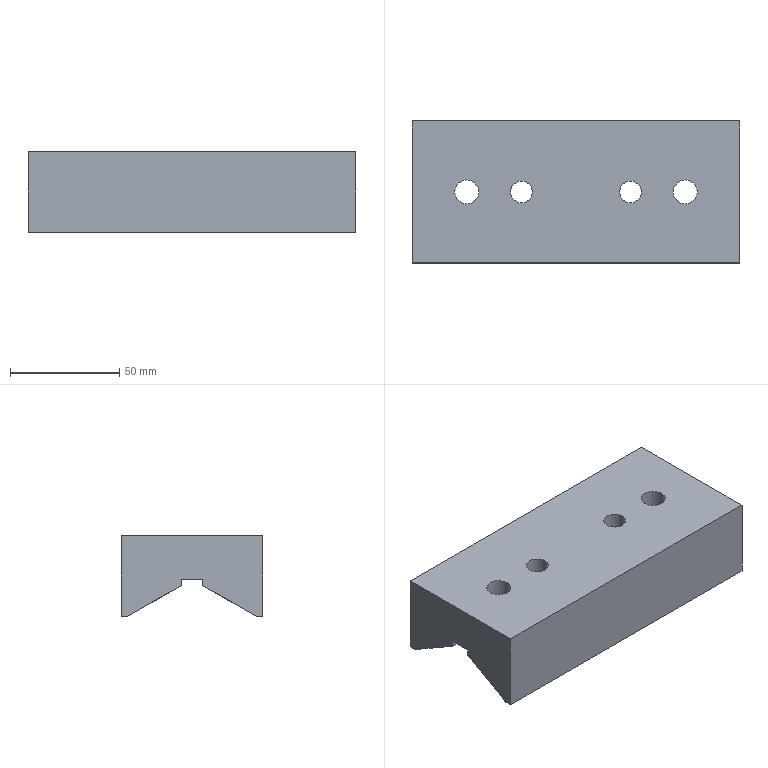Part | NX | features MAIN_BODY 2 | 1 solid | 34 faces | box 150 x 65 x 37 mm | volume 273059 mm3 | plane 24 | cylinder 10 | commonest cylinder face diameters 11 x6 10 x2 17.5 x2
STEP:
#1=CARTESIAN_POINT('',(625.,-5.,-355.));
#2=VERTEX_POINT('',#1);
#3=CARTESIAN_POINT('',(642.819,-5.,-355.));
#4=VERTEX_POINT('',#3);
#5=CARTESIAN_POINT('',(625.,-5.,-355.));
#6=DIRECTION('',(1.,0.,0.));
#7=VECTOR('',#6,1000.);
#8=LINE('',#5,#7);
#9=EDGE_CURVE('',#2,#4,#8,.T.);
#10=ORIENTED_EDGE('',*,*,#9,.F.);
#11=CARTESIAN_POINT('',(625.,5.,-355.));
#12=VERTEX_POINT('',#11);
#13=CARTESIAN_POINT('',(625.,5.,-355.));
#14=DIRECTION('',(0.,-1.,0.));
#15=VECTOR('',#14,1000.);
#16=LINE('',#13,#15);
#17=EDGE_CURVE('',#12,#2,#16,.T.);
#18=ORIENTED_EDGE('',*,*,#17,.F.);
#19=CARTESIAN_POINT('',(642.819,5.,-355.));
#20=VERTEX_POINT('',#19);
#21=CARTESIAN_POINT('',(625.,5.,-355.));
#22=DIRECTION('',(1.,0.,0.));
#23=VECTOR('',#22,1000.);
#24=LINE('',#21,#23);
#25=EDGE_CURVE('',#12,#20,#24,.T.);
#26=ORIENTED_EDGE('',*,*,#25,.T.);
#27=CARTESIAN_POINT('',(650.,0.,-355.));
#28=DIRECTION('',(0.,0.,-1.));
#29=DIRECTION('',(0.,-1.,0.));
#30=AXIS2_PLACEMENT_3D('',#27,#28,#29);
#31=CIRCLE('',#30,8.75);
#32=EDGE_CURVE('',#4,#20,#31,.T.);
#33=ORIENTED_EDGE('',*,*,#32,.F.);
#34=EDGE_LOOP('',(#10,#18,#26,#33));
#35=FACE_BOUND('',#34,.T.);
#36=CARTESIAN_POINT('',(625.,-5.,-355.));
#37=DIRECTION('',(0.,0.,1.));
#38=DIRECTION('',(0.,-1.,0.));
#39=AXIS2_PLACEMENT_3D('',#36,#37,#38);
#40=PLANE('',#39);
#41=ADVANCED_FACE('',(#35),#40,.F.);
#42=CARTESIAN_POINT('',(642.819,5.,-357.887));
#43=VERTEX_POINT('',#42);
#44=CARTESIAN_POINT('',(642.819,5.,-365.));
#45=DIRECTION('',(0.,0.,1.));
#46=VECTOR('',#45,1000.);
#47=LINE('',#44,#46);
#48=EDGE_CURVE('',#43,#20,#47,.T.);
#49=ORIENTED_EDGE('',*,*,#48,.T.);
#50=ORIENTED_EDGE('',*,*,#25,.F.);
#51=CARTESIAN_POINT('',(625.,5.,-357.887));
#52=VERTEX_POINT('',#51);
#53=CARTESIAN_POINT('',(625.,5.,-357.887));
#54=DIRECTION('',(0.,0.,1.));
#55=VECTOR('',#54,1000.);
#56=LINE('',#53,#55);
#57=EDGE_CURVE('',#52,#12,#56,.T.);
#58=ORIENTED_EDGE('',*,*,#57,.F.);
#59=CARTESIAN_POINT('',(625.,5.,-357.887));
#60=DIRECTION('',(1.,0.,0.));
#61=VECTOR('',#60,1000.);
#62=LINE('',#59,#61);
#63=EDGE_CURVE('',#52,#43,#62,.T.);
#64=ORIENTED_EDGE('',*,*,#63,.T.);
#65=EDGE_LOOP('',(#49,#50,#58,#64));
#66=FACE_BOUND('',#65,.T.);
#67=CARTESIAN_POINT('',(625.,5.,-357.887));
#68=DIRECTION('',(0.,-1.,0.));
#69=DIRECTION('',(0.,0.,-1.));
#70=AXIS2_PLACEMENT_3D('',#67,#68,#69);
#71=PLANE('',#70);
#72=ADVANCED_FACE('',(#66),#71,.T.);
#73=CARTESIAN_POINT('',(625.,-5.,-357.887));
#74=VERTEX_POINT('',#73);
#75=CARTESIAN_POINT('',(642.819,-5.,-357.887));
#76=VERTEX_POINT('',#75);
#77=CARTESIAN_POINT('',(625.,-5.,-357.887));
#78=DIRECTION('',(1.,0.,0.));
#79=VECTOR('',#78,1000.);
#80=LINE('',#77,#79);
#81=EDGE_CURVE('',#74,#76,#80,.T.);
#82=ORIENTED_EDGE('',*,*,#81,.F.);
#83=CARTESIAN_POINT('',(625.,-5.,-357.887));
#84=DIRECTION('',(0.,0.,1.));
#85=VECTOR('',#84,1000.);
#86=LINE('',#83,#85);
#87=EDGE_CURVE('',#74,#2,#86,.T.);
#88=ORIENTED_EDGE('',*,*,#87,.T.);
#89=ORIENTED_EDGE('',*,*,#9,.T.);
#90=CARTESIAN_POINT('',(642.819,-5.,-365.));
#91=DIRECTION('',(0.,0.,1.));
#92=VECTOR('',#91,1000.);
#93=LINE('',#90,#92);
#94=EDGE_CURVE('',#76,#4,#93,.T.);
#95=ORIENTED_EDGE('',*,*,#94,.F.);
#96=EDGE_LOOP('',(#82,#88,#89,#95));
#97=FACE_BOUND('',#96,.T.);
#98=CARTESIAN_POINT('',(625.,-5.,-357.887));
#99=DIRECTION('',(0.,-1.,0.));
#100=DIRECTION('',(0.,0.,-1.));
#101=AXIS2_PLACEMENT_3D('',#98,#99,#100);
#102=PLANE('',#101);
#103=ADVANCED_FACE('',(#97),#102,.F.);
#104=CARTESIAN_POINT('',(657.181,5.,-357.887));
#105=VERTEX_POINT('',#104);
#106=CARTESIAN_POINT('',(650.,0.,-355.));
#107=DIRECTION('',(0.,0.5,0.866));
#108=DIRECTION('',(0.,-0.866,0.5));
#109=AXIS2_PLACEMENT_3D('',#106,#107,#108);
#110=ELLIPSE('',#109,10.104,8.75);
#111=EDGE_CURVE('',#105,#43,#110,.T.);
#112=ORIENTED_EDGE('',*,*,#111,.T.);
#113=ORIENTED_EDGE('',*,*,#63,.F.);
#114=CARTESIAN_POINT('',(625.,29.445,-372.));
#115=VERTEX_POINT('',#114);
#116=CARTESIAN_POINT('',(625.,29.445,-372.));
#117=DIRECTION('',(0.,-0.866,0.5));
#118=VECTOR('',#117,1000.);
#119=LINE('',#116,#118);
#120=EDGE_CURVE('',#115,#52,#119,.T.);
#121=ORIENTED_EDGE('',*,*,#120,.F.);
#122=CARTESIAN_POINT('',(775.,29.445,-372.));
#123=VERTEX_POINT('',#122);
#124=CARTESIAN_POINT('',(625.,29.445,-372.));
#125=DIRECTION('',(1.,0.,0.));
#126=VECTOR('',#125,1000.);
#127=LINE('',#124,#126);
#128=EDGE_CURVE('',#115,#123,#127,.T.);
#129=ORIENTED_EDGE('',*,*,#128,.T.);
#130=CARTESIAN_POINT('',(775.,5.,-357.887));
#131=VERTEX_POINT('',#130);
#132=CARTESIAN_POINT('',(775.,29.445,-372.));
#133=DIRECTION('',(0.,-0.866,0.5));
#134=VECTOR('',#133,1000.);
#135=LINE('',#132,#134);
#136=EDGE_CURVE('',#123,#131,#135,.T.);
#137=ORIENTED_EDGE('',*,*,#136,.T.);
#138=CARTESIAN_POINT('',(757.181,5.,-357.887));
#139=VERTEX_POINT('',#138);
#140=CARTESIAN_POINT('',(625.,5.,-357.887));
#141=DIRECTION('',(1.,0.,0.));
#142=VECTOR('',#141,1000.);
#143=LINE('',#140,#142);
#144=EDGE_CURVE('',#139,#131,#143,.T.);
#145=ORIENTED_EDGE('',*,*,#144,.F.);
#146=CARTESIAN_POINT('',(742.819,5.,-357.887));
#147=VERTEX_POINT('',#146);
#148=CARTESIAN_POINT('',(750.,0.,-355.));
#149=DIRECTION('',(0.,0.5,0.866));
#150=DIRECTION('',(0.,-0.866,0.5));
#151=AXIS2_PLACEMENT_3D('',#148,#149,#150);
#152=ELLIPSE('',#151,10.104,8.75);
#153=EDGE_CURVE('',#147,#139,#152,.F.);
#154=ORIENTED_EDGE('',*,*,#153,.F.);
#155=CARTESIAN_POINT('',(727.291,5.,-357.887));
#156=VERTEX_POINT('',#155);
#157=CARTESIAN_POINT('',(625.,5.,-357.887));
#158=DIRECTION('',(1.,0.,0.));
#159=VECTOR('',#158,1000.);
#160=LINE('',#157,#159);
#161=EDGE_CURVE('',#156,#147,#160,.T.);
#162=ORIENTED_EDGE('',*,*,#161,.F.);
#163=CARTESIAN_POINT('',(722.709,5.,-357.887));
#164=VERTEX_POINT('',#163);
#165=CARTESIAN_POINT('',(725.,0.,-355.));
#166=DIRECTION('',(0.,0.5,0.866));
#167=DIRECTION('',(0.,0.866,-0.5));
#168=AXIS2_PLACEMENT_3D('',#165,#166,#167);
#169=ELLIPSE('',#168,6.351,5.5);
#170=EDGE_CURVE('',#164,#156,#169,.F.);
#171=ORIENTED_EDGE('',*,*,#170,.F.);
#172=CARTESIAN_POINT('',(677.291,5.,-357.887));
#173=VERTEX_POINT('',#172);
#174=CARTESIAN_POINT('',(625.,5.,-357.887));
#175=DIRECTION('',(1.,0.,0.));
#176=VECTOR('',#175,1000.);
#177=LINE('',#174,#176);
#178=EDGE_CURVE('',#173,#164,#177,.T.);
#179=ORIENTED_EDGE('',*,*,#178,.F.);
#180=CARTESIAN_POINT('',(672.709,5.,-357.887));
#181=VERTEX_POINT('',#180);
#182=CARTESIAN_POINT('',(675.,0.,-355.));
#183=DIRECTION('',(0.,0.5,0.866));
#184=DIRECTION('',(0.,0.866,-0.5));
#185=AXIS2_PLACEMENT_3D('',#182,#183,#184);
#186=ELLIPSE('',#185,6.351,5.5);
#187=EDGE_CURVE('',#181,#173,#186,.F.);
#188=ORIENTED_EDGE('',*,*,#187,.F.);
#189=CARTESIAN_POINT('',(625.,5.,-357.887));
#190=DIRECTION('',(1.,0.,0.));
#191=VECTOR('',#190,1000.);
#192=LINE('',#189,#191);
#193=EDGE_CURVE('',#105,#181,#192,.T.);
#194=ORIENTED_EDGE('',*,*,#193,.F.);
#195=EDGE_LOOP('',(#112,#113,#121,#129,#137,#145,#154,#162,#171,#179,#188,#194));
#196=FACE_BOUND('',#195,.T.);
#197=CARTESIAN_POINT('',(625.,29.445,-372.));
#198=DIRECTION('',(0.,-0.5,-0.866));
#199=DIRECTION('',(0.,0.866,-0.5));
#200=AXIS2_PLACEMENT_3D('',#197,#198,#199);
#201=PLANE('',#200);
#202=ADVANCED_FACE('',(#196),#201,.T.);
#203=CARTESIAN_POINT('',(727.291,5.,-355.));
#204=VERTEX_POINT('',#203);
#205=CARTESIAN_POINT('',(742.819,5.,-355.));
#206=VERTEX_POINT('',#205);
#207=CARTESIAN_POINT('',(625.,5.,-355.));
#208=DIRECTION('',(1.,0.,0.));
#209=VECTOR('',#208,1000.);
#210=LINE('',#207,#209);
#211=EDGE_CURVE('',#204,#206,#210,.T.);
#212=ORIENTED_EDGE('',*,*,#211,.F.);
#213=CARTESIAN_POINT('',(727.291,5.,-355.));
#214=DIRECTION('',(0.,0.,-1.));
#215=VECTOR('',#214,1000.);
#216=LINE('',#213,#215);
#217=EDGE_CURVE('',#156,#204,#216,.F.);
#218=ORIENTED_EDGE('',*,*,#217,.F.);
#219=ORIENTED_EDGE('',*,*,#161,.T.);
#220=CARTESIAN_POINT('',(742.819,5.,-365.));
#221=DIRECTION('',(0.,0.,1.));
#222=VECTOR('',#221,1000.);
#223=LINE('',#220,#222);
#224=EDGE_CURVE('',#206,#147,#223,.F.);
#225=ORIENTED_EDGE('',*,*,#224,.F.);
#226=EDGE_LOOP('',(#212,#218,#219,#225));
#227=FACE_BOUND('',#226,.T.);
#228=CARTESIAN_POINT('',(625.,5.,-357.887));
#229=DIRECTION('',(0.,-1.,0.));
#230=DIRECTION('',(0.,0.,-1.));
#231=AXIS2_PLACEMENT_3D('',#228,#229,#230);
#232=PLANE('',#231);
#233=ADVANCED_FACE('',(#227),#232,.T.);
#234=ORIENTED_EDGE('',*,*,#144,.T.);
#235=CARTESIAN_POINT('',(775.,5.,-355.));
#236=VERTEX_POINT('',#235);
#237=CARTESIAN_POINT('',(775.,5.,-357.887));
#238=DIRECTION('',(0.,0.,1.));
#239=VECTOR('',#238,1000.);
#240=LINE('',#237,#239);
#241=EDGE_CURVE('',#131,#236,#240,.T.);
#242=ORIENTED_EDGE('',*,*,#241,.T.);
#243=CARTESIAN_POINT('',(757.181,5.,-355.));
#244=VERTEX_POINT('',#243);
#245=CARTESIAN_POINT('',(625.,5.,-355.));
#246=DIRECTION('',(1.,0.,0.));
#247=VECTOR('',#246,1000.);
#248=LINE('',#245,#247);
#249=EDGE_CURVE('',#244,#236,#248,.T.);
#250=ORIENTED_EDGE('',*,*,#249,.F.);
#251=CARTESIAN_POINT('',(757.181,5.,-365.));
#252=DIRECTION('',(0.,0.,1.));
#253=VECTOR('',#252,1000.);
#254=LINE('',#251,#253);
#255=EDGE_CURVE('',#139,#244,#254,.T.);
#256=ORIENTED_EDGE('',*,*,#255,.F.);
#257=EDGE_LOOP('',(#234,#242,#250,#256));
#258=FACE_BOUND('',#257,.T.);
#259=CARTESIAN_POINT('',(625.,5.,-357.887));
#260=DIRECTION('',(0.,-1.,0.));
#261=DIRECTION('',(0.,0.,-1.));
#262=AXIS2_PLACEMENT_3D('',#259,#260,#261);
#263=PLANE('',#262);
#264=ADVANCED_FACE('',(#258),#263,.T.);
#265=CARTESIAN_POINT('',(742.819,-5.,-355.));
#266=VERTEX_POINT('',#265);
#267=CARTESIAN_POINT('',(742.819,-5.,-357.887));
#268=VERTEX_POINT('',#267);
#269=CARTESIAN_POINT('',(742.819,-5.,-365.));
#270=DIRECTION('',(0.,0.,1.));
#271=VECTOR('',#270,1000.);
#272=LINE('',#269,#271);
#273=EDGE_CURVE('',#266,#268,#272,.F.);
#274=ORIENTED_EDGE('',*,*,#273,.T.);
#275=CARTESIAN_POINT('',(727.291,-5.,-357.887));
#276=VERTEX_POINT('',#275);
#277=CARTESIAN_POINT('',(625.,-5.,-357.887));
#278=DIRECTION('',(1.,0.,0.));
#279=VECTOR('',#278,1000.);
#280=LINE('',#277,#279);
#281=EDGE_CURVE('',#276,#268,#280,.T.);
#282=ORIENTED_EDGE('',*,*,#281,.F.);
#283=CARTESIAN_POINT('',(727.291,-5.,-355.));
#284=VERTEX_POINT('',#283);
#285=CARTESIAN_POINT('',(727.291,-5.,-355.));
#286=DIRECTION('',(0.,0.,-1.));
#287=VECTOR('',#286,1000.);
#288=LINE('',#285,#287);
#289=EDGE_CURVE('',#276,#284,#288,.F.);
#290=ORIENTED_EDGE('',*,*,#289,.T.);
#291=CARTESIAN_POINT('',(625.,-5.,-355.));
#292=DIRECTION('',(1.,0.,0.));
#293=VECTOR('',#292,1000.);
#294=LINE('',#291,#293);
#295=EDGE_CURVE('',#284,#266,#294,.T.);
#296=ORIENTED_EDGE('',*,*,#295,.T.);
#297=EDGE_LOOP('',(#274,#282,#290,#296));
#298=FACE_BOUND('',#297,.T.);
#299=CARTESIAN_POINT('',(625.,-5.,-357.887));
#300=DIRECTION('',(0.,-1.,0.));
#301=DIRECTION('',(0.,0.,-1.));
#302=AXIS2_PLACEMENT_3D('',#299,#300,#301);
#303=PLANE('',#302);
#304=ADVANCED_FACE('',(#298),#303,.F.);
#305=CARTESIAN_POINT('',(757.181,-5.,-357.887));
#306=VERTEX_POINT('',#305);
#307=CARTESIAN_POINT('',(757.181,-5.,-355.));
#308=VERTEX_POINT('',#307);
#309=CARTESIAN_POINT('',(757.181,-5.,-365.));
#310=DIRECTION('',(0.,0.,1.));
#311=VECTOR('',#310,1000.);
#312=LINE('',#309,#311);
#313=EDGE_CURVE('',#306,#308,#312,.T.);
#314=ORIENTED_EDGE('',*,*,#313,.T.);
#315=CARTESIAN_POINT('',(775.,-5.,-355.));
#316=VERTEX_POINT('',#315);
#317=CARTESIAN_POINT('',(625.,-5.,-355.));
#318=DIRECTION('',(1.,0.,0.));
#319=VECTOR('',#318,1000.);
#320=LINE('',#317,#319);
#321=EDGE_CURVE('',#308,#316,#320,.T.);
#322=ORIENTED_EDGE('',*,*,#321,.T.);
#323=CARTESIAN_POINT('',(775.,-5.,-357.887));
#324=VERTEX_POINT('',#323);
#325=CARTESIAN_POINT('',(775.,-5.,-357.887));
#326=DIRECTION('',(0.,0.,1.));
#327=VECTOR('',#326,1000.);
#328=LINE('',#325,#327);
#329=EDGE_CURVE('',#324,#316,#328,.T.);
#330=ORIENTED_EDGE('',*,*,#329,.F.);
#331=CARTESIAN_POINT('',(625.,-5.,-357.887));
#332=DIRECTION('',(1.,0.,0.));
#333=VECTOR('',#332,1000.);
#334=LINE('',#331,#333);
#335=EDGE_CURVE('',#306,#324,#334,.T.);
#336=ORIENTED_EDGE('',*,*,#335,.F.);
#337=EDGE_LOOP('',(#314,#322,#330,#336));
#338=FACE_BOUND('',#337,.T.);
#339=CARTESIAN_POINT('',(625.,-5.,-357.887));
#340=DIRECTION('',(0.,-1.,0.));
#341=DIRECTION('',(0.,0.,-1.));
#342=AXIS2_PLACEMENT_3D('',#339,#340,#341);
#343=PLANE('',#342);
#344=ADVANCED_FACE('',(#338),#343,.F.);
#345=CARTESIAN_POINT('',(657.181,-5.,-357.887));
#346=VERTEX_POINT('',#345);
#347=CARTESIAN_POINT('',(672.709,-5.,-357.887));
#348=VERTEX_POINT('',#347);
#349=CARTESIAN_POINT('',(625.,-5.,-357.887));
#350=DIRECTION('',(1.,0.,0.));
#351=VECTOR('',#350,1000.);
#352=LINE('',#349,#351);
#353=EDGE_CURVE('',#346,#348,#352,.T.);
#354=ORIENTED_EDGE('',*,*,#353,.T.);
#355=CARTESIAN_POINT('',(677.291,-5.,-357.887));
#356=VERTEX_POINT('',#355);
#357=CARTESIAN_POINT('',(675.,0.,-355.));
#358=DIRECTION('',(0.,0.5,-0.866));
#359=DIRECTION('',(0.,-0.866,-0.5));
#360=AXIS2_PLACEMENT_3D('',#357,#358,#359);
#361=ELLIPSE('',#360,6.351,5.5);
#362=EDGE_CURVE('',#348,#356,#361,.F.);
#363=ORIENTED_EDGE('',*,*,#362,.T.);
#364=CARTESIAN_POINT('',(722.709,-5.,-357.887));
#365=VERTEX_POINT('',#364);
#366=CARTESIAN_POINT('',(625.,-5.,-357.887));
#367=DIRECTION('',(1.,0.,0.));
#368=VECTOR('',#367,1000.);
#369=LINE('',#366,#368);
#370=EDGE_CURVE('',#356,#365,#369,.T.);
#371=ORIENTED_EDGE('',*,*,#370,.T.);
#372=CARTESIAN_POINT('',(725.,0.,-355.));
#373=DIRECTION('',(0.,0.5,-0.866));
#374=DIRECTION('',(0.,-0.866,-0.5));
#375=AXIS2_PLACEMENT_3D('',#372,#373,#374);
#376=ELLIPSE('',#375,6.351,5.5);
#377=EDGE_CURVE('',#365,#276,#376,.F.);
#378=ORIENTED_EDGE('',*,*,#377,.T.);
#379=ORIENTED_EDGE('',*,*,#281,.T.);
#380=CARTESIAN_POINT('',(750.,0.,-355.));
#381=DIRECTION('',(0.,0.5,-0.866));
#382=DIRECTION('',(0.,0.866,0.5));
#383=AXIS2_PLACEMENT_3D('',#380,#381,#382);
#384=ELLIPSE('',#383,10.104,8.75);
#385=EDGE_CURVE('',#268,#306,#384,.F.);
#386=ORIENTED_EDGE('',*,*,#385,.T.);
#387=ORIENTED_EDGE('',*,*,#335,.T.);
#388=CARTESIAN_POINT('',(775.,-29.445,-372.));
#389=VERTEX_POINT('',#388);
#390=CARTESIAN_POINT('',(775.,-29.445,-372.));
#391=DIRECTION('',(0.,0.866,0.5));
#392=VECTOR('',#391,1000.);
#393=LINE('',#390,#392);
#394=EDGE_CURVE('',#389,#324,#393,.T.);
#395=ORIENTED_EDGE('',*,*,#394,.F.);
#396=CARTESIAN_POINT('',(625.,-29.445,-372.));
#397=VERTEX_POINT('',#396);
#398=CARTESIAN_POINT('',(625.,-29.445,-372.));
#399=DIRECTION('',(1.,0.,0.));
#400=VECTOR('',#399,1000.);
#401=LINE('',#398,#400);
#402=EDGE_CURVE('',#397,#389,#401,.T.);
#403=ORIENTED_EDGE('',*,*,#402,.F.);
#404=CARTESIAN_POINT('',(625.,-29.445,-372.));
#405=DIRECTION('',(0.,0.866,0.5));
#406=VECTOR('',#405,1000.);
#407=LINE('',#404,#406);
#408=EDGE_CURVE('',#397,#74,#407,.T.);
#409=ORIENTED_EDGE('',*,*,#408,.T.);
#410=ORIENTED_EDGE('',*,*,#81,.T.);
#411=CARTESIAN_POINT('',(650.,0.,-355.));
#412=DIRECTION('',(0.,0.5,-0.866));
#413=DIRECTION('',(0.,0.866,0.5));
#414=AXIS2_PLACEMENT_3D('',#411,#412,#413);
#415=ELLIPSE('',#414,10.104,8.75);
#416=EDGE_CURVE('',#346,#76,#415,.T.);
#417=ORIENTED_EDGE('',*,*,#416,.F.);
#418=EDGE_LOOP('',(#354,#363,#371,#378,#379,#386,#387,#395,#403,#409,#410,#417));
#419=FACE_BOUND('',#418,.T.);
#420=CARTESIAN_POINT('',(625.,-29.445,-372.));
#421=DIRECTION('',(0.,-0.5,0.866));
#422=DIRECTION('',(0.,-0.866,-0.5));
#423=AXIS2_PLACEMENT_3D('',#420,#421,#422);
#424=PLANE('',#423);
#425=ADVANCED_FACE('',(#419),#424,.F.);
#426=CARTESIAN_POINT('',(750.,0.,-355.));
#427=DIRECTION('',(0.,0.,-1.));
#428=DIRECTION('',(0.,-1.,0.));
#429=AXIS2_PLACEMENT_3D('',#426,#427,#428);
#430=CIRCLE('',#429,8.75);
#431=EDGE_CURVE('',#308,#244,#430,.F.);
#432=ORIENTED_EDGE('',*,*,#431,.T.);
#433=ORIENTED_EDGE('',*,*,#249,.T.);
#434=CARTESIAN_POINT('',(775.,-5.,-355.));
#435=DIRECTION('',(0.,1.,0.));
#436=VECTOR('',#435,1000.);
#437=LINE('',#434,#436);
#438=EDGE_CURVE('',#316,#236,#437,.T.);
#439=ORIENTED_EDGE('',*,*,#438,.F.);
#440=ORIENTED_EDGE('',*,*,#321,.F.);
#441=EDGE_LOOP('',(#432,#433,#439,#440));
#442=FACE_BOUND('',#441,.T.);
#443=CARTESIAN_POINT('',(625.,-5.,-355.));
#444=DIRECTION('',(0.,0.,1.));
#445=DIRECTION('',(0.,-1.,0.));
#446=AXIS2_PLACEMENT_3D('',#443,#444,#445);
#447=PLANE('',#446);
#448=ADVANCED_FACE('',(#442),#447,.F.);
#449=CARTESIAN_POINT('',(675.,5.,-355.));
#450=VERTEX_POINT('',#449);
#451=CARTESIAN_POINT('',(675.,0.,-355.));
#452=DIRECTION('',(0.,0.,1.));
#453=DIRECTION('',(0.,1.,0.));
#454=AXIS2_PLACEMENT_3D('',#451,#452,#453);
#455=CIRCLE('',#454,5.);
#456=EDGE_CURVE('',#450,#450,#455,.T.);
#457=ORIENTED_EDGE('',*,*,#456,.T.);
#458=EDGE_LOOP('',(#457));
#459=FACE_BOUND('',#458,.T.);
#460=CARTESIAN_POINT('',(725.,5.,-355.));
#461=VERTEX_POINT('',#460);
#462=CARTESIAN_POINT('',(725.,0.,-355.));
#463=DIRECTION('',(0.,0.,1.));
#464=DIRECTION('',(0.,1.,0.));
#465=AXIS2_PLACEMENT_3D('',#462,#463,#464);
#466=CIRCLE('',#465,5.);
#467=EDGE_CURVE('',#461,#461,#466,.T.);
#468=ORIENTED_EDGE('',*,*,#467,.T.);
#469=EDGE_LOOP('',(#468));
#470=FACE_BOUND('',#469,.T.);
#471=CARTESIAN_POINT('',(657.181,5.,-355.));
#472=VERTEX_POINT('',#471);
#473=CARTESIAN_POINT('',(672.709,5.,-355.));
#474=VERTEX_POINT('',#473);
#475=CARTESIAN_POINT('',(625.,5.,-355.));
#476=DIRECTION('',(1.,0.,0.));
#477=VECTOR('',#476,1000.);
#478=LINE('',#475,#477);
#479=EDGE_CURVE('',#472,#474,#478,.T.);
#480=ORIENTED_EDGE('',*,*,#479,.T.);
#481=CARTESIAN_POINT('',(677.291,5.,-355.));
#482=VERTEX_POINT('',#481);
#483=CARTESIAN_POINT('',(675.,0.,-355.));
#484=DIRECTION('',(0.,0.,1.));
#485=DIRECTION('',(0.,1.,0.));
#486=AXIS2_PLACEMENT_3D('',#483,#484,#485);
#487=CIRCLE('',#486,5.5);
#488=EDGE_CURVE('',#474,#482,#487,.F.);
#489=ORIENTED_EDGE('',*,*,#488,.T.);
#490=CARTESIAN_POINT('',(722.709,5.,-355.));
#491=VERTEX_POINT('',#490);
#492=CARTESIAN_POINT('',(625.,5.,-355.));
#493=DIRECTION('',(1.,0.,0.));
#494=VECTOR('',#493,1000.);
#495=LINE('',#492,#494);
#496=EDGE_CURVE('',#482,#491,#495,.T.);
#497=ORIENTED_EDGE('',*,*,#496,.T.);
#498=CARTESIAN_POINT('',(725.,0.,-355.));
#499=DIRECTION('',(0.,0.,1.));
#500=DIRECTION('',(0.,1.,0.));
#501=AXIS2_PLACEMENT_3D('',#498,#499,#500);
#502=CIRCLE('',#501,5.5);
#503=EDGE_CURVE('',#491,#204,#502,.F.);
#504=ORIENTED_EDGE('',*,*,#503,.T.);
#505=ORIENTED_EDGE('',*,*,#211,.T.);
#506=CARTESIAN_POINT('',(750.,0.,-355.));
#507=DIRECTION('',(0.,0.,-1.));
#508=DIRECTION('',(0.,-1.,0.));
#509=AXIS2_PLACEMENT_3D('',#506,#507,#508);
#510=CIRCLE('',#509,8.75);
#511=EDGE_CURVE('',#206,#266,#510,.F.);
#512=ORIENTED_EDGE('',*,*,#511,.T.);
#513=ORIENTED_EDGE('',*,*,#295,.F.);
#514=CARTESIAN_POINT('',(722.709,-5.,-355.));
#515=VERTEX_POINT('',#514);
#516=CARTESIAN_POINT('',(725.,0.,-355.));
#517=DIRECTION('',(0.,0.,1.));
#518=DIRECTION('',(0.,1.,0.));
#519=AXIS2_PLACEMENT_3D('',#516,#517,#518);
#520=CIRCLE('',#519,5.5);
#521=EDGE_CURVE('',#284,#515,#520,.F.);
#522=ORIENTED_EDGE('',*,*,#521,.T.);
#523=CARTESIAN_POINT('',(677.291,-5.,-355.));
#524=VERTEX_POINT('',#523);
#525=CARTESIAN_POINT('',(625.,-5.,-355.));
#526=DIRECTION('',(1.,0.,0.));
#527=VECTOR('',#526,1000.);
#528=LINE('',#525,#527);
#529=EDGE_CURVE('',#524,#515,#528,.T.);
#530=ORIENTED_EDGE('',*,*,#529,.F.);
#531=CARTESIAN_POINT('',(672.709,-5.,-355.));
#532=VERTEX_POINT('',#531);
#533=CARTESIAN_POINT('',(675.,0.,-355.));
#534=DIRECTION('',(0.,0.,1.));
#535=DIRECTION('',(0.,1.,0.));
#536=AXIS2_PLACEMENT_3D('',#533,#534,#535);
#537=CIRCLE('',#536,5.5);
#538=EDGE_CURVE('',#524,#532,#537,.F.);
#539=ORIENTED_EDGE('',*,*,#538,.T.);
#540=CARTESIAN_POINT('',(657.181,-5.,-355.));
#541=VERTEX_POINT('',#540);
#542=CARTESIAN_POINT('',(625.,-5.,-355.));
#543=DIRECTION('',(1.,0.,0.));
#544=VECTOR('',#543,1000.);
#545=LINE('',#542,#544);
#546=EDGE_CURVE('',#541,#532,#545,.T.);
#547=ORIENTED_EDGE('',*,*,#546,.F.);
#548=CARTESIAN_POINT('',(650.,0.,-355.));
#549=DIRECTION('',(0.,0.,-1.));
#550=DIRECTION('',(0.,-1.,0.));
#551=AXIS2_PLACEMENT_3D('',#548,#549,#550);
#552=CIRCLE('',#551,8.75);
#553=EDGE_CURVE('',#472,#541,#552,.T.);
#554=ORIENTED_EDGE('',*,*,#553,.F.);
#555=EDGE_LOOP('',(#480,#489,#497,#504,#505,#512,#513,#522,#530,#539,#547,#554));
#556=FACE_BOUND('',#555,.T.);
#557=CARTESIAN_POINT('',(625.,-5.,-355.));
#558=DIRECTION('',(0.,0.,1.));
#559=DIRECTION('',(0.,-1.,0.));
#560=AXIS2_PLACEMENT_3D('',#557,#558,#559);
#561=PLANE('',#560);
#562=ADVANCED_FACE('',(#459,#470,#556),#561,.F.);
#563=CARTESIAN_POINT('',(650.,5.5,-335.));
#564=VERTEX_POINT('',#563);
#565=CARTESIAN_POINT('',(650.,0.,-335.));
#566=DIRECTION('',(0.,0.,-1.));
#567=DIRECTION('',(0.,1.,0.));
#568=AXIS2_PLACEMENT_3D('',#565,#566,#567);
#569=CIRCLE('',#568,5.5);
#570=EDGE_CURVE('',#564,#564,#569,.T.);
#571=ORIENTED_EDGE('',*,*,#570,.T.);
#572=EDGE_LOOP('',(#571));
#573=FACE_BOUND('',#572,.T.);
#574=CARTESIAN_POINT('',(775.,-32.5,-335.));
#575=VERTEX_POINT('',#574);
#576=CARTESIAN_POINT('',(775.,32.5,-335.));
#577=VERTEX_POINT('',#576);
#578=CARTESIAN_POINT('',(775.,0.,-335.));
#579=DIRECTION('',(0.,1.,0.));
#580=VECTOR('',#579,1000.);
#581=LINE('',#578,#580);
#582=EDGE_CURVE('',#575,#577,#581,.T.);
#583=ORIENTED_EDGE('',*,*,#582,.T.);
#584=CARTESIAN_POINT('',(625.,32.5,-335.));
#585=VERTEX_POINT('',#584);
#586=CARTESIAN_POINT('',(625.,32.5,-335.));
#587=DIRECTION('',(1.,0.,0.));
#588=VECTOR('',#587,1000.);
#589=LINE('',#586,#588);
#590=EDGE_CURVE('',#585,#577,#589,.T.);
#591=ORIENTED_EDGE('',*,*,#590,.F.);
#592=CARTESIAN_POINT('',(625.,-32.5,-335.));
#593=VERTEX_POINT('',#592);
#594=CARTESIAN_POINT('',(625.,0.,-335.));
#595=DIRECTION('',(0.,-1.,0.));
#596=VECTOR('',#595,1000.);
#597=LINE('',#594,#596);
#598=EDGE_CURVE('',#585,#593,#597,.T.);
#599=ORIENTED_EDGE('',*,*,#598,.T.);
#600=CARTESIAN_POINT('',(625.,-32.5,-335.));
#601=DIRECTION('',(1.,0.,0.));
#602=VECTOR('',#601,1000.);
#603=LINE('',#600,#602);
#604=EDGE_CURVE('',#593,#575,#603,.T.);
#605=ORIENTED_EDGE('',*,*,#604,.T.);
#606=EDGE_LOOP('',(#583,#591,#599,#605));
#607=FACE_BOUND('',#606,.T.);
#608=CARTESIAN_POINT('',(675.,5.,-335.));
#609=VERTEX_POINT('',#608);
#610=CARTESIAN_POINT('',(675.,0.,-335.));
#611=DIRECTION('',(0.,0.,1.));
#612=DIRECTION('',(0.,1.,0.));
#613=AXIS2_PLACEMENT_3D('',#610,#611,#612);
#614=CIRCLE('',#613,5.);
#615=EDGE_CURVE('',#609,#609,#614,.T.);
#616=ORIENTED_EDGE('',*,*,#615,.F.);
#617=EDGE_LOOP('',(#616));
#618=FACE_BOUND('',#617,.T.);
#619=CARTESIAN_POINT('',(725.,5.,-335.));
#620=VERTEX_POINT('',#619);
#621=CARTESIAN_POINT('',(725.,0.,-335.));
#622=DIRECTION('',(0.,0.,1.));
#623=DIRECTION('',(0.,1.,0.));
#624=AXIS2_PLACEMENT_3D('',#621,#622,#623);
#625=CIRCLE('',#624,5.);
#626=EDGE_CURVE('',#620,#620,#625,.T.);
#627=ORIENTED_EDGE('',*,*,#626,.F.);
#628=EDGE_LOOP('',(#627));
#629=FACE_BOUND('',#628,.T.);
#630=CARTESIAN_POINT('',(750.,5.5,-335.));
#631=VERTEX_POINT('',#630);
#632=CARTESIAN_POINT('',(750.,0.,-335.));
#633=DIRECTION('',(0.,0.,1.));
#634=DIRECTION('',(0.,1.,0.));
#635=AXIS2_PLACEMENT_3D('',#632,#633,#634);
#636=CIRCLE('',#635,5.5);
#637=EDGE_CURVE('',#631,#631,#636,.T.);
#638=ORIENTED_EDGE('',*,*,#637,.F.);
#639=EDGE_LOOP('',(#638));
#640=FACE_BOUND('',#639,.T.);
#641=CARTESIAN_POINT('',(625.,0.,-335.));
#642=DIRECTION('',(0.,0.,1.));
#643=DIRECTION('',(0.,-1.,0.));
#644=AXIS2_PLACEMENT_3D('',#641,#642,#643);
#645=PLANE('',#644);
#646=ADVANCED_FACE('',(#573,#607,#618,#629,#640),#645,.T.);
#647=ORIENTED_EDGE('',*,*,#496,.F.);
#648=CARTESIAN_POINT('',(677.291,5.,-355.));
#649=DIRECTION('',(0.,0.,-1.));
#650=VECTOR('',#649,1000.);
#651=LINE('',#648,#650);
#652=EDGE_CURVE('',#173,#482,#651,.F.);
#653=ORIENTED_EDGE('',*,*,#652,.F.);
#654=ORIENTED_EDGE('',*,*,#178,.T.);
#655=CARTESIAN_POINT('',(722.709,5.,-355.));
#656=DIRECTION('',(0.,0.,-1.));
#657=VECTOR('',#656,1000.);
#658=LINE('',#655,#657);
#659=EDGE_CURVE('',#491,#164,#658,.T.);
#660=ORIENTED_EDGE('',*,*,#659,.F.);
#661=EDGE_LOOP('',(#647,#653,#654,#660));
#662=FACE_BOUND('',#661,.T.);
#663=CARTESIAN_POINT('',(625.,5.,-357.887));
#664=DIRECTION('',(0.,-1.,0.));
#665=DIRECTION('',(0.,0.,-1.));
#666=AXIS2_PLACEMENT_3D('',#663,#664,#665);
#667=PLANE('',#666);
#668=ADVANCED_FACE('',(#662),#667,.T.);
#669=CARTESIAN_POINT('',(722.709,-5.,-355.));
#670=DIRECTION('',(0.,0.,-1.));
#671=VECTOR('',#670,1000.);
#672=LINE('',#669,#671);
#673=EDGE_CURVE('',#515,#365,#672,.T.);
#674=ORIENTED_EDGE('',*,*,#673,.T.);
#675=ORIENTED_EDGE('',*,*,#370,.F.);
#676=CARTESIAN_POINT('',(677.291,-5.,-355.));
#677=DIRECTION('',(0.,0.,-1.));
#678=VECTOR('',#677,1000.);
#679=LINE('',#676,#678);
#680=EDGE_CURVE('',#356,#524,#679,.F.);
#681=ORIENTED_EDGE('',*,*,#680,.T.);
#682=ORIENTED_EDGE('',*,*,#529,.T.);
#683=EDGE_LOOP('',(#674,#675,#681,#682));
#684=FACE_BOUND('',#683,.T.);
#685=CARTESIAN_POINT('',(625.,-5.,-357.887));
#686=DIRECTION('',(0.,-1.,0.));
#687=DIRECTION('',(0.,0.,-1.));
#688=AXIS2_PLACEMENT_3D('',#685,#686,#687);
#689=PLANE('',#688);
#690=ADVANCED_FACE('',(#684),#689,.F.);
#691=CARTESIAN_POINT('',(657.181,5.,-365.));
#692=DIRECTION('',(0.,0.,1.));
#693=VECTOR('',#692,1000.);
#694=LINE('',#691,#693);
#695=EDGE_CURVE('',#472,#105,#694,.F.);
#696=ORIENTED_EDGE('',*,*,#695,.T.);
#697=ORIENTED_EDGE('',*,*,#193,.T.);
#698=CARTESIAN_POINT('',(672.709,5.,-355.));
#699=DIRECTION('',(0.,0.,-1.));
#700=VECTOR('',#699,1000.);
#701=LINE('',#698,#700);
#702=EDGE_CURVE('',#474,#181,#701,.T.);
#703=ORIENTED_EDGE('',*,*,#702,.F.);
#704=ORIENTED_EDGE('',*,*,#479,.F.);
#705=EDGE_LOOP('',(#696,#697,#703,#704));
#706=FACE_BOUND('',#705,.T.);
#707=CARTESIAN_POINT('',(625.,5.,-357.887));
#708=DIRECTION('',(0.,-1.,0.));
#709=DIRECTION('',(0.,0.,-1.));
#710=AXIS2_PLACEMENT_3D('',#707,#708,#709);
#711=PLANE('',#710);
#712=ADVANCED_FACE('',(#706),#711,.T.);
#713=ORIENTED_EDGE('',*,*,#546,.T.);
#714=CARTESIAN_POINT('',(672.709,-5.,-355.));
#715=DIRECTION('',(0.,0.,-1.));
#716=VECTOR('',#715,1000.);
#717=LINE('',#714,#716);
#718=EDGE_CURVE('',#532,#348,#717,.T.);
#719=ORIENTED_EDGE('',*,*,#718,.T.);
#720=ORIENTED_EDGE('',*,*,#353,.F.);
#721=CARTESIAN_POINT('',(657.181,-5.,-365.));
#722=DIRECTION('',(0.,0.,1.));
#723=VECTOR('',#722,1000.);
#724=LINE('',#721,#723);
#725=EDGE_CURVE('',#541,#346,#724,.F.);
#726=ORIENTED_EDGE('',*,*,#725,.F.);
#727=EDGE_LOOP('',(#713,#719,#720,#726));
#728=FACE_BOUND('',#727,.T.);
#729=CARTESIAN_POINT('',(625.,-5.,-357.887));
#730=DIRECTION('',(0.,-1.,0.));
#731=DIRECTION('',(0.,0.,-1.));
#732=AXIS2_PLACEMENT_3D('',#729,#730,#731);
#733=PLANE('',#732);
#734=ADVANCED_FACE('',(#728),#733,.F.);
#735=CARTESIAN_POINT('',(775.,32.5,-372.));
#736=VERTEX_POINT('',#735);
#737=CARTESIAN_POINT('',(775.,32.5,-372.));
#738=DIRECTION('',(0.,-1.,0.));
#739=VECTOR('',#738,1000.);
#740=LINE('',#737,#739);
#741=EDGE_CURVE('',#736,#123,#740,.T.);
#742=ORIENTED_EDGE('',*,*,#741,.T.);
#743=ORIENTED_EDGE('',*,*,#128,.F.);
#744=CARTESIAN_POINT('',(625.,32.5,-372.));
#745=VERTEX_POINT('',#744);
#746=CARTESIAN_POINT('',(625.,32.5,-372.));
#747=DIRECTION('',(0.,-1.,0.));
#748=VECTOR('',#747,1000.);
#749=LINE('',#746,#748);
#750=EDGE_CURVE('',#745,#115,#749,.T.);
#751=ORIENTED_EDGE('',*,*,#750,.F.);
#752=CARTESIAN_POINT('',(625.,32.5,-372.));
#753=DIRECTION('',(1.,0.,0.));
#754=VECTOR('',#753,1000.);
#755=LINE('',#752,#754);
#756=EDGE_CURVE('',#745,#736,#755,.T.);
#757=ORIENTED_EDGE('',*,*,#756,.T.);
#758=EDGE_LOOP('',(#742,#743,#751,#757));
#759=FACE_BOUND('',#758,.T.);
#760=CARTESIAN_POINT('',(625.,32.5,-372.));
#761=DIRECTION('',(0.,0.,-1.));
#762=DIRECTION('',(0.,1.,0.));
#763=AXIS2_PLACEMENT_3D('',#760,#761,#762);
#764=PLANE('',#763);
#765=ADVANCED_FACE('',(#759),#764,.T.);
#766=CARTESIAN_POINT('',(775.,-32.5,-372.));
#767=VERTEX_POINT('',#766);
#768=CARTESIAN_POINT('',(775.,-32.5,-372.));
#769=DIRECTION('',(0.,1.,0.));
#770=VECTOR('',#769,1000.);
#771=LINE('',#768,#770);
#772=EDGE_CURVE('',#767,#389,#771,.T.);
#773=ORIENTED_EDGE('',*,*,#772,.F.);
#774=CARTESIAN_POINT('',(625.,-32.5,-372.));
#775=VERTEX_POINT('',#774);
#776=CARTESIAN_POINT('',(625.,-32.5,-372.));
#777=DIRECTION('',(1.,0.,0.));
#778=VECTOR('',#777,1000.);
#779=LINE('',#776,#778);
#780=EDGE_CURVE('',#775,#767,#779,.T.);
#781=ORIENTED_EDGE('',*,*,#780,.F.);
#782=CARTESIAN_POINT('',(625.,-32.5,-372.));
#783=DIRECTION('',(0.,1.,0.));
#784=VECTOR('',#783,1000.);
#785=LINE('',#782,#784);
#786=EDGE_CURVE('',#775,#397,#785,.T.);
#787=ORIENTED_EDGE('',*,*,#786,.T.);
#788=ORIENTED_EDGE('',*,*,#402,.T.);
#789=EDGE_LOOP('',(#773,#781,#787,#788));
#790=FACE_BOUND('',#789,.T.);
#791=CARTESIAN_POINT('',(625.,-32.5,-372.));
#792=DIRECTION('',(0.,0.,1.));
#793=DIRECTION('',(0.,-1.,0.));
#794=AXIS2_PLACEMENT_3D('',#791,#792,#793);
#795=PLANE('',#794);
#796=ADVANCED_FACE('',(#790),#795,.F.);
#797=CARTESIAN_POINT('',(775.,-32.5,-335.));
#798=DIRECTION('',(0.,0.,-1.));
#799=VECTOR('',#798,1000.);
#800=LINE('',#797,#799);
#801=EDGE_CURVE('',#575,#767,#800,.T.);
#802=ORIENTED_EDGE('',*,*,#801,.F.);
#803=ORIENTED_EDGE('',*,*,#604,.F.);
#804=CARTESIAN_POINT('',(625.,-32.5,-335.));
#805=DIRECTION('',(0.,0.,-1.));
#806=VECTOR('',#805,1000.);
#807=LINE('',#804,#806);
#808=EDGE_CURVE('',#593,#775,#807,.T.);
#809=ORIENTED_EDGE('',*,*,#808,.T.);
#810=ORIENTED_EDGE('',*,*,#780,.T.);
#811=EDGE_LOOP('',(#802,#803,#809,#810));
#812=FACE_BOUND('',#811,.T.);
#813=CARTESIAN_POINT('',(625.,-32.5,-335.));
#814=DIRECTION('',(0.,1.,0.));
#815=DIRECTION('',(0.,0.,1.));
#816=AXIS2_PLACEMENT_3D('',#813,#814,#815);
#817=PLANE('',#816);
#818=ADVANCED_FACE('',(#812),#817,.F.);
#819=CARTESIAN_POINT('',(775.,32.5,-335.));
#820=DIRECTION('',(0.,0.,-1.));
#821=VECTOR('',#820,1000.);
#822=LINE('',#819,#821);
#823=EDGE_CURVE('',#577,#736,#822,.T.);
#824=ORIENTED_EDGE('',*,*,#823,.T.);
#825=ORIENTED_EDGE('',*,*,#756,.F.);
#826=CARTESIAN_POINT('',(625.,32.5,-335.));
#827=DIRECTION('',(0.,0.,-1.));
#828=VECTOR('',#827,1000.);
#829=LINE('',#826,#828);
#830=EDGE_CURVE('',#585,#745,#829,.T.);
#831=ORIENTED_EDGE('',*,*,#830,.F.);
#832=ORIENTED_EDGE('',*,*,#590,.T.);
#833=EDGE_LOOP('',(#824,#825,#831,#832));
#834=FACE_BOUND('',#833,.T.);
#835=CARTESIAN_POINT('',(625.,32.5,-335.));
#836=DIRECTION('',(0.,1.,0.));
#837=DIRECTION('',(0.,0.,1.));
#838=AXIS2_PLACEMENT_3D('',#835,#836,#837);
#839=PLANE('',#838);
#840=ADVANCED_FACE('',(#834),#839,.T.);
#841=ORIENTED_EDGE('',*,*,#750,.T.);
#842=ORIENTED_EDGE('',*,*,#120,.T.);
#843=ORIENTED_EDGE('',*,*,#57,.T.);
#844=ORIENTED_EDGE('',*,*,#17,.T.);
#845=ORIENTED_EDGE('',*,*,#87,.F.);
#846=ORIENTED_EDGE('',*,*,#408,.F.);
#847=ORIENTED_EDGE('',*,*,#786,.F.);
#848=ORIENTED_EDGE('',*,*,#808,.F.);
#849=ORIENTED_EDGE('',*,*,#598,.F.);
#850=ORIENTED_EDGE('',*,*,#830,.T.);
#851=EDGE_LOOP('',(#841,#842,#843,#844,#845,#846,#847,#848,#849,#850));
#852=FACE_BOUND('',#851,.T.);
#853=CARTESIAN_POINT('',(625.,-32.5,-372.));
#854=DIRECTION('',(-1.,0.,0.));
#855=DIRECTION('',(0.,0.,-1.));
#856=AXIS2_PLACEMENT_3D('',#853,#854,#855);
#857=PLANE('',#856);
#858=ADVANCED_FACE('',(#852),#857,.T.);
#859=ORIENTED_EDGE('',*,*,#741,.F.);
#860=ORIENTED_EDGE('',*,*,#823,.F.);
#861=ORIENTED_EDGE('',*,*,#582,.F.);
#862=ORIENTED_EDGE('',*,*,#801,.T.);
#863=ORIENTED_EDGE('',*,*,#772,.T.);
#864=ORIENTED_EDGE('',*,*,#394,.T.);
#865=ORIENTED_EDGE('',*,*,#329,.T.);
#866=ORIENTED_EDGE('',*,*,#438,.T.);
#867=ORIENTED_EDGE('',*,*,#241,.F.);
#868=ORIENTED_EDGE('',*,*,#136,.F.);
#869=EDGE_LOOP('',(#859,#860,#861,#862,#863,#864,#865,#866,#867,#868));
#870=FACE_BOUND('',#869,.T.);
#871=CARTESIAN_POINT('',(775.,-32.5,-372.));
#872=DIRECTION('',(-1.,0.,0.));
#873=DIRECTION('',(0.,0.,-1.));
#874=AXIS2_PLACEMENT_3D('',#871,#872,#873);
#875=PLANE('',#874);
#876=ADVANCED_FACE('',(#870),#875,.F.);
#877=ORIENTED_EDGE('',*,*,#456,.F.);
#878=EDGE_LOOP('',(#877));
#879=FACE_BOUND('',#878,.T.);
#880=ORIENTED_EDGE('',*,*,#615,.T.);
#881=EDGE_LOOP('',(#880));
#882=FACE_BOUND('',#881,.T.);
#883=CARTESIAN_POINT('',(675.,0.,-335.));
#884=DIRECTION('',(0.,0.,-1.));
#885=DIRECTION('',(0.,1.,0.));
#886=AXIS2_PLACEMENT_3D('',#883,#884,#885);
#887=CYLINDRICAL_SURFACE('',#886,5.);
#888=ADVANCED_FACE('',(#879,#882),#887,.F.);
#889=ORIENTED_EDGE('',*,*,#467,.F.);
#890=EDGE_LOOP('',(#889));
#891=FACE_BOUND('',#890,.T.);
#892=ORIENTED_EDGE('',*,*,#626,.T.);
#893=EDGE_LOOP('',(#892));
#894=FACE_BOUND('',#893,.T.);
#895=CARTESIAN_POINT('',(725.,0.,-335.));
#896=DIRECTION('',(0.,0.,-1.));
#897=DIRECTION('',(0.,1.,0.));
#898=AXIS2_PLACEMENT_3D('',#895,#896,#897);
#899=CYLINDRICAL_SURFACE('',#898,5.);
#900=ADVANCED_FACE('',(#891,#894),#899,.F.);
#901=ORIENTED_EDGE('',*,*,#680,.F.);
#902=ORIENTED_EDGE('',*,*,#362,.F.);
#903=ORIENTED_EDGE('',*,*,#718,.F.);
#904=ORIENTED_EDGE('',*,*,#538,.F.);
#905=EDGE_LOOP('',(#901,#902,#903,#904));
#906=FACE_BOUND('',#905,.T.);
#907=CARTESIAN_POINT('',(675.,0.,-355.));
#908=DIRECTION('',(0.,0.,-1.));
#909=DIRECTION('',(0.,1.,0.));
#910=AXIS2_PLACEMENT_3D('',#907,#908,#909);
#911=CYLINDRICAL_SURFACE('',#910,5.5);
#912=ADVANCED_FACE('',(#906),#911,.F.);
#913=ORIENTED_EDGE('',*,*,#187,.T.);
#914=ORIENTED_EDGE('',*,*,#652,.T.);
#915=ORIENTED_EDGE('',*,*,#488,.F.);
#916=ORIENTED_EDGE('',*,*,#702,.T.);
#917=EDGE_LOOP('',(#913,#914,#915,#916));
#918=FACE_BOUND('',#917,.T.);
#919=CARTESIAN_POINT('',(675.,0.,-355.));
#920=DIRECTION('',(0.,0.,-1.));
#921=DIRECTION('',(0.,1.,0.));
#922=AXIS2_PLACEMENT_3D('',#919,#920,#921);
#923=CYLINDRICAL_SURFACE('',#922,5.5);
#924=ADVANCED_FACE('',(#918),#923,.F.);
#925=ORIENTED_EDGE('',*,*,#289,.F.);
#926=ORIENTED_EDGE('',*,*,#377,.F.);
#927=ORIENTED_EDGE('',*,*,#673,.F.);
#928=ORIENTED_EDGE('',*,*,#521,.F.);
#929=EDGE_LOOP('',(#925,#926,#927,#928));
#930=FACE_BOUND('',#929,.T.);
#931=CARTESIAN_POINT('',(725.,0.,-355.));
#932=DIRECTION('',(0.,0.,-1.));
#933=DIRECTION('',(0.,1.,0.));
#934=AXIS2_PLACEMENT_3D('',#931,#932,#933);
#935=CYLINDRICAL_SURFACE('',#934,5.5);
#936=ADVANCED_FACE('',(#930),#935,.F.);
#937=ORIENTED_EDGE('',*,*,#170,.T.);
#938=ORIENTED_EDGE('',*,*,#217,.T.);
#939=ORIENTED_EDGE('',*,*,#503,.F.);
#940=ORIENTED_EDGE('',*,*,#659,.T.);
#941=EDGE_LOOP('',(#937,#938,#939,#940));
#942=FACE_BOUND('',#941,.T.);
#943=CARTESIAN_POINT('',(725.,0.,-355.));
#944=DIRECTION('',(0.,0.,-1.));
#945=DIRECTION('',(0.,1.,0.));
#946=AXIS2_PLACEMENT_3D('',#943,#944,#945);
#947=CYLINDRICAL_SURFACE('',#946,5.5);
#948=ADVANCED_FACE('',(#942),#947,.F.);
#949=CARTESIAN_POINT('',(750.,5.5,-345.));
#950=VERTEX_POINT('',#949);
#951=CARTESIAN_POINT('',(750.,0.,-345.));
#952=DIRECTION('',(0.,0.,1.));
#953=DIRECTION('',(0.,1.,0.));
#954=AXIS2_PLACEMENT_3D('',#951,#952,#953);
#955=CIRCLE('',#954,5.5);
#956=EDGE_CURVE('',#950,#950,#955,.T.);
#957=ORIENTED_EDGE('',*,*,#956,.F.);
#958=EDGE_LOOP('',(#957));
#959=FACE_BOUND('',#958,.T.);
#960=ORIENTED_EDGE('',*,*,#637,.T.);
#961=EDGE_LOOP('',(#960));
#962=FACE_BOUND('',#961,.T.);
#963=CARTESIAN_POINT('',(750.,0.,-345.));
#964=DIRECTION('',(0.,0.,1.));
#965=DIRECTION('',(0.,-1.,0.));
#966=AXIS2_PLACEMENT_3D('',#963,#964,#965);
#967=CYLINDRICAL_SURFACE('',#966,5.5);
#968=ADVANCED_FACE('',(#959,#962),#967,.F.);
#969=CARTESIAN_POINT('',(650.,-5.5,-345.));
#970=VERTEX_POINT('',#969);
#971=CARTESIAN_POINT('',(650.,0.,-345.));
#972=DIRECTION('',(0.,0.,-1.));
#973=DIRECTION('',(0.,-1.,0.));
#974=AXIS2_PLACEMENT_3D('',#971,#972,#973);
#975=CIRCLE('',#974,5.5);
#976=EDGE_CURVE('',#970,#970,#975,.F.);
#977=ORIENTED_EDGE('',*,*,#976,.F.);
#978=EDGE_LOOP('',(#977));
#979=FACE_BOUND('',#978,.T.);
#980=ORIENTED_EDGE('',*,*,#570,.F.);
#981=EDGE_LOOP('',(#980));
#982=FACE_BOUND('',#981,.T.);
#983=CARTESIAN_POINT('',(650.,0.,-345.));
#984=DIRECTION('',(0.,0.,1.));
#985=DIRECTION('',(0.,-1.,0.));
#986=AXIS2_PLACEMENT_3D('',#983,#984,#985);
#987=CYLINDRICAL_SURFACE('',#986,5.5);
#988=ADVANCED_FACE('',(#979,#982),#987,.F.);
#989=CARTESIAN_POINT('',(750.,8.75,-345.));
#990=VERTEX_POINT('',#989);
#991=CARTESIAN_POINT('',(750.,0.,-345.));
#992=DIRECTION('',(0.,0.,1.));
#993=DIRECTION('',(0.,1.,0.));
#994=AXIS2_PLACEMENT_3D('',#991,#992,#993);
#995=CIRCLE('',#994,8.75);
#996=EDGE_CURVE('',#990,#990,#995,.T.);
#997=ORIENTED_EDGE('',*,*,#996,.T.);
#998=EDGE_LOOP('',(#997));
#999=FACE_BOUND('',#998,.T.);
#1000=ORIENTED_EDGE('',*,*,#431,.F.);
#1001=ORIENTED_EDGE('',*,*,#313,.F.);
#1002=ORIENTED_EDGE('',*,*,#385,.F.);
#1003=ORIENTED_EDGE('',*,*,#273,.F.);
#1004=ORIENTED_EDGE('',*,*,#511,.F.);
#1005=ORIENTED_EDGE('',*,*,#224,.T.);
#1006=ORIENTED_EDGE('',*,*,#153,.T.);
#1007=ORIENTED_EDGE('',*,*,#255,.T.);
#1008=EDGE_LOOP('',(#1000,#1001,#1002,#1003,#1004,#1005,#1006,#1007));
#1009=FACE_BOUND('',#1008,.T.);
#1010=CARTESIAN_POINT('',(750.,0.,-365.));
#1011=DIRECTION('',(0.,0.,1.));
#1012=DIRECTION('',(0.,-1.,0.));
#1013=AXIS2_PLACEMENT_3D('',#1010,#1011,#1012);
#1014=CYLINDRICAL_SURFACE('',#1013,8.75);
#1015=ADVANCED_FACE('',(#999,#1009),#1014,.F.);
#1016=ORIENTED_EDGE('',*,*,#956,.T.);
#1017=EDGE_LOOP('',(#1016));
#1018=FACE_BOUND('',#1017,.T.);
#1019=ORIENTED_EDGE('',*,*,#996,.F.);
#1020=EDGE_LOOP('',(#1019));
#1021=FACE_BOUND('',#1020,.T.);
#1022=CARTESIAN_POINT('',(750.,0.,-345.));
#1023=DIRECTION('',(0.,0.,-1.));
#1024=DIRECTION('',(0.,1.,0.));
#1025=AXIS2_PLACEMENT_3D('',#1022,#1023,#1024);
#1026=PLANE('',#1025);
#1027=ADVANCED_FACE('',(#1018,#1021),#1026,.T.);
#1028=CARTESIAN_POINT('',(650.,8.75,-345.));
#1029=VERTEX_POINT('',#1028);
#1030=CARTESIAN_POINT('',(650.,0.,-345.));
#1031=DIRECTION('',(0.,0.,-1.));
#1032=DIRECTION('',(0.,1.,0.));
#1033=AXIS2_PLACEMENT_3D('',#1030,#1031,#1032);
#1034=CIRCLE('',#1033,8.75);
#1035=EDGE_CURVE('',#1029,#1029,#1034,.T.);
#1036=ORIENTED_EDGE('',*,*,#1035,.T.);
#1037=EDGE_LOOP('',(#1036));
#1038=FACE_BOUND('',#1037,.T.);
#1039=ORIENTED_EDGE('',*,*,#976,.T.);
#1040=EDGE_LOOP('',(#1039));
#1041=FACE_BOUND('',#1040,.T.);
#1042=CARTESIAN_POINT('',(650.,0.,-345.));
#1043=DIRECTION('',(0.,0.,1.));
#1044=DIRECTION('',(0.,-1.,0.));
#1045=AXIS2_PLACEMENT_3D('',#1042,#1043,#1044);
#1046=PLANE('',#1045);
#1047=ADVANCED_FACE('',(#1038,#1041),#1046,.F.);
#1048=ORIENTED_EDGE('',*,*,#48,.F.);
#1049=ORIENTED_EDGE('',*,*,#111,.F.);
#1050=ORIENTED_EDGE('',*,*,#695,.F.);
#1051=ORIENTED_EDGE('',*,*,#553,.T.);
#1052=ORIENTED_EDGE('',*,*,#725,.T.);
#1053=ORIENTED_EDGE('',*,*,#416,.T.);
#1054=ORIENTED_EDGE('',*,*,#94,.T.);
#1055=ORIENTED_EDGE('',*,*,#32,.T.);
#1056=EDGE_LOOP('',(#1048,#1049,#1050,#1051,#1052,#1053,#1054,#1055));
#1057=FACE_BOUND('',#1056,.T.);
#1058=ORIENTED_EDGE('',*,*,#1035,.F.);
#1059=EDGE_LOOP('',(#1058));
#1060=FACE_BOUND('',#1059,.T.);
#1061=CARTESIAN_POINT('',(650.,0.,-365.));
#1062=DIRECTION('',(0.,0.,1.));
#1063=DIRECTION('',(0.,-1.,0.));
#1064=AXIS2_PLACEMENT_3D('',#1061,#1062,#1063);
#1065=CYLINDRICAL_SURFACE('',#1064,8.75);
#1066=ADVANCED_FACE('',(#1057,#1060),#1065,.F.);
#1067=CLOSED_SHELL('',(#41,#72,#103,#202,#233,#264,#304,#344,#425,#448,#562,#646,#668,#690,#712,#734,#765,#796,#818,#840,#858,#876,#888,#900,#912,#924,#936,#948,#968,#988,#1015,#1027,#1047,#1066));
#1068=MANIFOLD_SOLID_BREP('',#1067);
#1069=(LENGTH_UNIT()NAMED_UNIT(*)SI_UNIT(.MILLI.,.METRE.));
#1070=UNCERTAINTY_MEASURE_WITH_UNIT(LENGTH_MEASURE(0.00001),#1069,'','');
#1071=(NAMED_UNIT(*)PLANE_ANGLE_UNIT()SI_UNIT($,.RADIAN.));
#1072=(NAMED_UNIT(*)SI_UNIT($,.STERADIAN.)SOLID_ANGLE_UNIT());
#1073=(GEOMETRIC_REPRESENTATION_CONTEXT(3)GLOBAL_UNCERTAINTY_ASSIGNED_CONTEXT((#1070))GLOBAL_UNIT_ASSIGNED_CONTEXT((#1069,#1071,#1072))REPRESENTATION_CONTEXT('',''));
#1074=ADVANCED_BREP_SHAPE_REPRESENTATION('',(#1068),#1073);